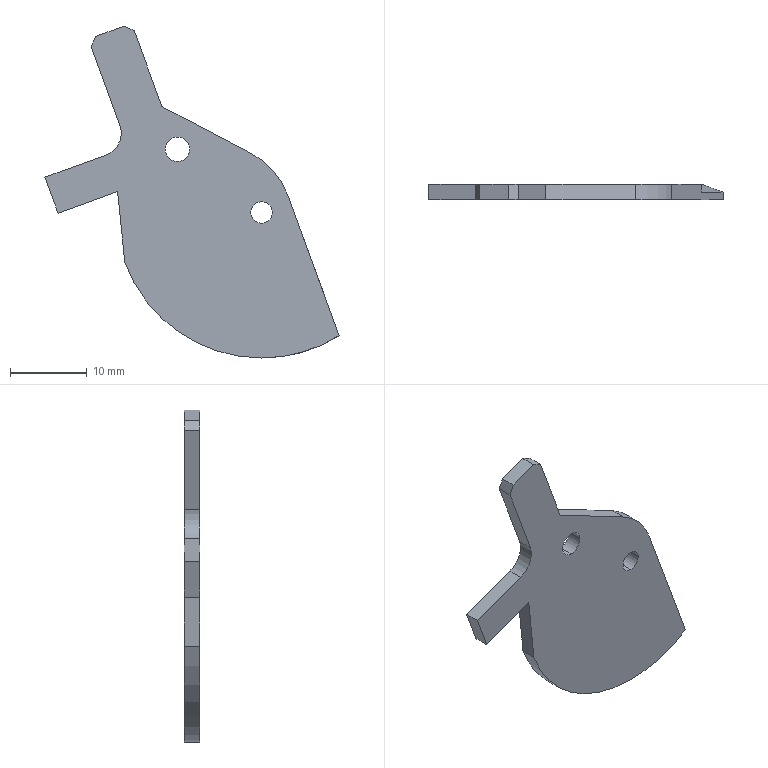Part | SolidWorks | features ICE 14, Fillet 4, Chamfer 3, Extrusion 1 | 1 solid | 23 faces | box 38.392 x 2 x 43.344 mm | volume 1473 mm3 | plane 15 | cylinder 8 | commonest cylinder face diameters 2.8 x2 3.2 x2 38 x2 6 x1 20 x1
STEP:
#1=CARTESIAN_POINT('',(-10.981,0.,6.641));
#2=VERTEX_POINT('',#1);
#3=CARTESIAN_POINT('',(-10.981,0.,9.841));
#4=VERTEX_POINT('',#3);
#5=CARTESIAN_POINT('',(-10.981,0.,8.241));
#6=DIRECTION('',(0.,1.,0.));
#7=DIRECTION('',(0.,0.,1.));
#8=AXIS2_PLACEMENT_3D('',#5,#6,#7);
#9=CIRCLE('',#8,1.6);
#10=EDGE_CURVE('',#2,#4,#9,.T.);
#11=ORIENTED_EDGE('',*,*,#10,.F.);
#12=CARTESIAN_POINT('',(-10.981,2.,6.641));
#13=VERTEX_POINT('',#12);
#14=CARTESIAN_POINT('',(-10.981,-8.,6.641));
#15=DIRECTION('',(0.,1.,0.));
#16=VECTOR('',#15,1000.);
#17=LINE('',#14,#16);
#18=EDGE_CURVE('',#2,#13,#17,.T.);
#19=ORIENTED_EDGE('',*,*,#18,.T.);
#20=CARTESIAN_POINT('',(-10.981,2.,9.841));
#21=VERTEX_POINT('',#20);
#22=CARTESIAN_POINT('',(-10.981,2.,8.241));
#23=DIRECTION('',(0.,1.,0.));
#24=DIRECTION('',(0.,0.,1.));
#25=AXIS2_PLACEMENT_3D('',#22,#23,#24);
#26=CIRCLE('',#25,1.6);
#27=EDGE_CURVE('',#13,#21,#26,.T.);
#28=ORIENTED_EDGE('',*,*,#27,.T.);
#29=CARTESIAN_POINT('',(-10.981,-8.,9.841));
#30=DIRECTION('',(0.,1.,0.));
#31=VECTOR('',#30,1000.);
#32=LINE('',#29,#31);
#33=EDGE_CURVE('',#4,#21,#32,.T.);
#34=ORIENTED_EDGE('',*,*,#33,.F.);
#35=EDGE_LOOP('',(#11,#19,#28,#34));
#36=FACE_OUTER_BOUND('',#35,.T.);
#37=CARTESIAN_POINT('',(-10.981,-8.,8.241));
#38=DIRECTION('',(0.,1.,0.));
#39=DIRECTION('',(0.,0.,1.));
#40=AXIS2_PLACEMENT_3D('',#37,#38,#39);
#41=CYLINDRICAL_SURFACE('',#40,1.6);
#42=ADVANCED_FACE('',(#36),#41,.F.);
#43=CARTESIAN_POINT('',(0.,0.,-1.4));
#44=VERTEX_POINT('',#43);
#45=CARTESIAN_POINT('',(0.,0.,1.4));
#46=VERTEX_POINT('',#45);
#47=CARTESIAN_POINT('',(0.,0.,0.));
#48=DIRECTION('',(0.,1.,0.));
#49=DIRECTION('',(0.,0.,1.));
#50=AXIS2_PLACEMENT_3D('',#47,#48,#49);
#51=CIRCLE('',#50,1.4);
#52=EDGE_CURVE('',#44,#46,#51,.T.);
#53=ORIENTED_EDGE('',*,*,#52,.F.);
#54=CARTESIAN_POINT('',(0.,2.,-1.4));
#55=VERTEX_POINT('',#54);
#56=CARTESIAN_POINT('',(0.,-3.,-1.4));
#57=DIRECTION('',(0.,1.,0.));
#58=VECTOR('',#57,1000.);
#59=LINE('',#56,#58);
#60=EDGE_CURVE('',#44,#55,#59,.T.);
#61=ORIENTED_EDGE('',*,*,#60,.T.);
#62=CARTESIAN_POINT('',(0.,2.,1.4));
#63=VERTEX_POINT('',#62);
#64=CARTESIAN_POINT('',(0.,2.,0.));
#65=DIRECTION('',(0.,1.,0.));
#66=DIRECTION('',(0.,0.,1.));
#67=AXIS2_PLACEMENT_3D('',#64,#65,#66);
#68=CIRCLE('',#67,1.4);
#69=EDGE_CURVE('',#55,#63,#68,.T.);
#70=ORIENTED_EDGE('',*,*,#69,.T.);
#71=CARTESIAN_POINT('',(0.,-3.,1.4));
#72=DIRECTION('',(0.,1.,0.));
#73=VECTOR('',#72,1000.);
#74=LINE('',#71,#73);
#75=EDGE_CURVE('',#46,#63,#74,.T.);
#76=ORIENTED_EDGE('',*,*,#75,.F.);
#77=EDGE_LOOP('',(#53,#61,#70,#76));
#78=FACE_OUTER_BOUND('',#77,.T.);
#79=CARTESIAN_POINT('',(0.,-3.,0.));
#80=DIRECTION('',(0.,1.,0.));
#81=DIRECTION('',(0.,0.,1.));
#82=AXIS2_PLACEMENT_3D('',#79,#80,#81);
#83=CYLINDRICAL_SURFACE('',#82,1.4);
#84=ADVANCED_FACE('',(#78),#83,.F.);
#85=CARTESIAN_POINT('',(0.,2.,-19.));
#86=VERTEX_POINT('',#85);
#87=CARTESIAN_POINT('',(-17.854,2.,-6.498));
#88=VERTEX_POINT('',#87);
#89=CARTESIAN_POINT('',(0.,2.,0.));
#90=DIRECTION('',(0.,1.,0.));
#91=DIRECTION('',(0.,0.,1.));
#92=AXIS2_PLACEMENT_3D('',#89,#90,#91);
#93=CIRCLE('',#92,19.);
#94=EDGE_CURVE('',#86,#88,#93,.T.);
#95=ORIENTED_EDGE('',*,*,#94,.F.);
#96=CARTESIAN_POINT('',(0.,0.,-19.));
#97=VERTEX_POINT('',#96);
#98=CARTESIAN_POINT('',(0.,2.,-19.));
#99=DIRECTION('',(0.,-1.,0.));
#100=VECTOR('',#99,1000.);
#101=LINE('',#98,#100);
#102=EDGE_CURVE('',#86,#97,#101,.T.);
#103=ORIENTED_EDGE('',*,*,#102,.T.);
#104=CARTESIAN_POINT('',(-17.854,0.,-6.498));
#105=VERTEX_POINT('',#104);
#106=CARTESIAN_POINT('',(0.,0.,0.));
#107=DIRECTION('',(0.,1.,0.));
#108=DIRECTION('',(0.,0.,1.));
#109=AXIS2_PLACEMENT_3D('',#106,#107,#108);
#110=CIRCLE('',#109,19.);
#111=EDGE_CURVE('',#97,#105,#110,.T.);
#112=ORIENTED_EDGE('',*,*,#111,.T.);
#113=CARTESIAN_POINT('',(-17.854,-8.,-6.498));
#114=DIRECTION('',(0.,1.,0.));
#115=VECTOR('',#114,1000.);
#116=LINE('',#113,#115);
#117=EDGE_CURVE('',#105,#88,#116,.T.);
#118=ORIENTED_EDGE('',*,*,#117,.T.);
#119=EDGE_LOOP('',(#95,#103,#112,#118));
#120=FACE_OUTER_BOUND('',#119,.T.);
#121=CARTESIAN_POINT('',(0.,2.,0.));
#122=DIRECTION('',(0.,-1.,0.));
#123=DIRECTION('',(0.,0.,-1.));
#124=AXIS2_PLACEMENT_3D('',#121,#122,#123);
#125=CYLINDRICAL_SURFACE('',#124,19.);
#126=ADVANCED_FACE('',(#120),#125,.T.);
#127=ORIENTED_EDGE('',*,*,#102,.F.);
#128=CARTESIAN_POINT('',(7.429,2.,-17.487));
#129=VERTEX_POINT('',#128);
#130=CARTESIAN_POINT('',(0.,2.,0.));
#131=DIRECTION('',(0.,1.,0.));
#132=DIRECTION('',(0.,0.,1.));
#133=AXIS2_PLACEMENT_3D('',#130,#131,#132);
#134=CIRCLE('',#133,19.);
#135=EDGE_CURVE('',#129,#86,#134,.T.);
#136=ORIENTED_EDGE('',*,*,#135,.F.);
#137=CARTESIAN_POINT('',(10.112,1.,-16.086));
#138=VERTEX_POINT('',#137);
#139=CARTESIAN_POINT('',(7.429,2.,-17.487));
#140=CARTESIAN_POINT('',(8.36,1.663,-17.092));
#141=CARTESIAN_POINT('',(9.256,1.329,-16.624));
#142=CARTESIAN_POINT('',(10.112,1.,-16.086));
#143=(BOUNDED_CURVE()B_SPLINE_CURVE(3,(#139,#140,#141,#142),.UNSPECIFIED.,.F.,.F.)B_SPLINE_CURVE_WITH_KNOTS((4,4),(4.765,4.925),.UNSPECIFIED.)CURVE()GEOMETRIC_REPRESENTATION_ITEM()RATIONAL_B_SPLINE_CURVE((1.,0.9979,0.9979,1.))REPRESENTATION_ITEM(''));
#144=EDGE_CURVE('',#129,#138,#143,.T.);
#145=ORIENTED_EDGE('',*,*,#144,.T.);
#146=CARTESIAN_POINT('',(10.112,0.,-16.086));
#147=VERTEX_POINT('',#146);
#148=CARTESIAN_POINT('',(10.112,2.,-16.086));
#149=DIRECTION('',(0.,-1.,0.));
#150=VECTOR('',#149,1000.);
#151=LINE('',#148,#150);
#152=EDGE_CURVE('',#138,#147,#151,.T.);
#153=ORIENTED_EDGE('',*,*,#152,.T.);
#154=CARTESIAN_POINT('',(0.,0.,0.));
#155=DIRECTION('',(0.,1.,0.));
#156=DIRECTION('',(0.,0.,1.));
#157=AXIS2_PLACEMENT_3D('',#154,#155,#156);
#158=CIRCLE('',#157,19.);
#159=EDGE_CURVE('',#147,#97,#158,.T.);
#160=ORIENTED_EDGE('',*,*,#159,.T.);
#161=EDGE_LOOP('',(#127,#136,#145,#153,#160));
#162=FACE_OUTER_BOUND('',#161,.T.);
#163=CARTESIAN_POINT('',(0.,2.,0.));
#164=DIRECTION('',(0.,-1.,0.));
#165=DIRECTION('',(0.,0.,-1.));
#166=AXIS2_PLACEMENT_3D('',#163,#164,#165);
#167=CYLINDRICAL_SURFACE('',#166,19.);
#168=ADVANCED_FACE('',(#162),#167,.T.);
#169=CARTESIAN_POINT('',(-10.981,2.,8.241));
#170=DIRECTION('',(0.,1.,0.));
#171=DIRECTION('',(0.,0.,1.));
#172=AXIS2_PLACEMENT_3D('',#169,#170,#171);
#173=CIRCLE('',#172,1.6);
#174=EDGE_CURVE('',#21,#13,#173,.T.);
#175=ORIENTED_EDGE('',*,*,#174,.F.);
#176=ORIENTED_EDGE('',*,*,#27,.F.);
#177=EDGE_LOOP('',(#175,#176));
#178=FACE_BOUND('',#177,.T.);
#179=CARTESIAN_POINT('',(-21.665,2.,22.976));
#180=VERTEX_POINT('',#179);
#181=CARTESIAN_POINT('',(-17.906,2.,24.344));
#182=VERTEX_POINT('',#181);
#183=CARTESIAN_POINT('',(-16.966,2.,24.686));
#184=DIRECTION('',(0.9397,0.,0.342));
#185=VECTOR('',#184,1000.);
#186=LINE('',#183,#185);
#187=EDGE_CURVE('',#180,#182,#186,.T.);
#188=ORIENTED_EDGE('',*,*,#187,.T.);
#189=CARTESIAN_POINT('',(-16.624,2.,23.746));
#190=VERTEX_POINT('',#189);
#191=CARTESIAN_POINT('',(6.126,2.,13.138));
#192=DIRECTION('',(0.9063,0.,-0.4226));
#193=VECTOR('',#192,1000.);
#194=LINE('',#191,#193);
#195=EDGE_CURVE('',#182,#190,#194,.T.);
#196=ORIENTED_EDGE('',*,*,#195,.T.);
#197=CARTESIAN_POINT('',(-13.018,2.,13.839));
#198=VERTEX_POINT('',#197);
#199=CARTESIAN_POINT('',(-10.126,2.,5.892));
#200=DIRECTION('',(0.342,0.,-0.9397));
#201=VECTOR('',#200,1000.);
#202=LINE('',#199,#201);
#203=EDGE_CURVE('',#190,#198,#202,.T.);
#204=ORIENTED_EDGE('',*,*,#203,.T.);
#205=CARTESIAN_POINT('',(-1.306,2.,7.682));
#206=VERTEX_POINT('',#205);
#207=CARTESIAN_POINT('',(-13.018,2.,13.839));
#208=DIRECTION('',(-0.8851,0.,0.4653));
#209=VECTOR('',#208,1000.);
#210=LINE('',#207,#209);
#211=EDGE_CURVE('',#206,#198,#210,.T.);
#212=ORIENTED_EDGE('',*,*,#211,.F.);
#213=CARTESIAN_POINT('',(3.437,2.,2.251));
#214=VERTEX_POINT('',#213);
#215=CARTESIAN_POINT('',(-5.96,2.,-1.169));
#216=DIRECTION('',(0.,1.,0.));
#217=DIRECTION('',(0.,0.,1.));
#218=AXIS2_PLACEMENT_3D('',#215,#216,#217);
#219=CIRCLE('',#218,10.);
#220=EDGE_CURVE('',#206,#214,#219,.T.);
#221=ORIENTED_EDGE('',*,*,#220,.T.);
#222=CARTESIAN_POINT('',(7.261,2.,-8.256));
#223=VERTEX_POINT('',#222);
#224=CARTESIAN_POINT('',(-2.999,2.,19.935));
#225=DIRECTION('',(0.342,0.,-0.9397));
#226=VECTOR('',#225,1000.);
#227=LINE('',#224,#226);
#228=EDGE_CURVE('',#214,#223,#227,.T.);
#229=ORIENTED_EDGE('',*,*,#228,.T.);
#230=CARTESIAN_POINT('',(4.442,2.,-9.282));
#231=VERTEX_POINT('',#230);
#232=CARTESIAN_POINT('',(7.261,2.,-8.256));
#233=DIRECTION('',(-0.9397,0.,-0.342));
#234=VECTOR('',#233,1000.);
#235=LINE('',#232,#234);
#236=EDGE_CURVE('',#223,#231,#235,.T.);
#237=ORIENTED_EDGE('',*,*,#236,.T.);
#238=CARTESIAN_POINT('',(7.292,2.,-17.112));
#239=DIRECTION('',(0.342,0.,-0.9397));
#240=VECTOR('',#239,1000.);
#241=LINE('',#238,#240);
#242=EDGE_CURVE('',#231,#129,#241,.T.);
#243=ORIENTED_EDGE('',*,*,#242,.T.);
#244=ORIENTED_EDGE('',*,*,#135,.T.);
#245=ORIENTED_EDGE('',*,*,#94,.T.);
#246=CARTESIAN_POINT('',(-18.802,2.,2.734));
#247=VERTEX_POINT('',#246);
#248=CARTESIAN_POINT('',(-18.802,2.,2.734));
#249=DIRECTION('',(0.1022,0.,-0.9948));
#250=VECTOR('',#249,1000.);
#251=LINE('',#248,#250);
#252=EDGE_CURVE('',#247,#88,#251,.T.);
#253=ORIENTED_EDGE('',*,*,#252,.F.);
#254=CARTESIAN_POINT('',(-26.57,2.,-0.09327));
#255=VERTEX_POINT('',#254);
#256=CARTESIAN_POINT('',(-26.57,2.,-0.09327));
#257=DIRECTION('',(-0.9397,0.,-0.342));
#258=VECTOR('',#257,1000.);
#259=LINE('',#256,#258);
#260=EDGE_CURVE('',#247,#255,#259,.T.);
#261=ORIENTED_EDGE('',*,*,#260,.T.);
#262=CARTESIAN_POINT('',(-28.281,2.,4.605));
#263=VERTEX_POINT('',#262);
#264=CARTESIAN_POINT('',(-28.281,2.,4.605));
#265=DIRECTION('',(-0.342,0.,0.9397));
#266=VECTOR('',#265,1000.);
#267=LINE('',#264,#266);
#268=EDGE_CURVE('',#255,#263,#267,.T.);
#269=ORIENTED_EDGE('',*,*,#268,.T.);
#270=CARTESIAN_POINT('',(-20.293,2.,7.512));
#271=VERTEX_POINT('',#270);
#272=CARTESIAN_POINT('',(-17.474,2.,8.538));
#273=DIRECTION('',(0.9397,0.,0.342));
#274=VECTOR('',#273,1000.);
#275=LINE('',#272,#274);
#276=EDGE_CURVE('',#263,#271,#275,.T.);
#277=ORIENTED_EDGE('',*,*,#276,.T.);
#278=CARTESIAN_POINT('',(-18.5,2.,11.358));
#279=VERTEX_POINT('',#278);
#280=CARTESIAN_POINT('',(-21.319,2.,10.331));
#281=DIRECTION('',(0.,-1.,0.));
#282=DIRECTION('',(0.,0.,1.));
#283=AXIS2_PLACEMENT_3D('',#280,#281,#282);
#284=CIRCLE('',#283,3.);
#285=EDGE_CURVE('',#271,#279,#284,.T.);
#286=ORIENTED_EDGE('',*,*,#285,.T.);
#287=CARTESIAN_POINT('',(-22.262,2.,21.694));
#288=VERTEX_POINT('',#287);
#289=CARTESIAN_POINT('',(-22.604,2.,22.634));
#290=DIRECTION('',(-0.342,0.,0.9397));
#291=VECTOR('',#290,1000.);
#292=LINE('',#289,#291);
#293=EDGE_CURVE('',#279,#288,#292,.T.);
#294=ORIENTED_EDGE('',*,*,#293,.T.);
#295=CARTESIAN_POINT('',(-26.596,2.,12.402));
#296=DIRECTION('',(0.4226,0.,0.9063));
#297=VECTOR('',#296,1000.);
#298=LINE('',#295,#297);
#299=EDGE_CURVE('',#288,#180,#298,.T.);
#300=ORIENTED_EDGE('',*,*,#299,.T.);
#301=EDGE_LOOP('',(#188,#196,#204,#212,#221,#229,#237,#243,#244,#245,#253,#261,#269,#277,#286,#294,#300));
#302=FACE_OUTER_BOUND('',#301,.T.);
#303=CARTESIAN_POINT('',(0.,2.,0.));
#304=DIRECTION('',(0.,1.,0.));
#305=DIRECTION('',(0.,0.,1.));
#306=AXIS2_PLACEMENT_3D('',#303,#304,#305);
#307=CIRCLE('',#306,1.4);
#308=EDGE_CURVE('',#63,#55,#307,.T.);
#309=ORIENTED_EDGE('',*,*,#308,.F.);
#310=ORIENTED_EDGE('',*,*,#69,.F.);
#311=EDGE_LOOP('',(#309,#310));
#312=FACE_BOUND('',#311,.T.);
#313=CARTESIAN_POINT('',(0.,2.,0.));
#314=DIRECTION('',(0.,1.,0.));
#315=DIRECTION('',(0.,0.,1.));
#316=AXIS2_PLACEMENT_3D('',#313,#314,#315);
#317=PLANE('',#316);
#318=ADVANCED_FACE('',(#178,#302,#312),#317,.T.);
#319=CARTESIAN_POINT('',(-10.981,0.,8.241));
#320=DIRECTION('',(0.,1.,0.));
#321=DIRECTION('',(0.,0.,1.));
#322=AXIS2_PLACEMENT_3D('',#319,#320,#321);
#323=CIRCLE('',#322,1.6);
#324=EDGE_CURVE('',#4,#2,#323,.T.);
#325=ORIENTED_EDGE('',*,*,#324,.T.);
#326=ORIENTED_EDGE('',*,*,#10,.T.);
#327=EDGE_LOOP('',(#325,#326));
#328=FACE_BOUND('',#327,.T.);
#329=CARTESIAN_POINT('',(-13.018,0.,13.839));
#330=VERTEX_POINT('',#329);
#331=CARTESIAN_POINT('',(-16.624,0.,23.746));
#332=VERTEX_POINT('',#331);
#333=CARTESIAN_POINT('',(-10.126,0.,5.892));
#334=DIRECTION('',(-0.342,0.,0.9397));
#335=VECTOR('',#334,1000.);
#336=LINE('',#333,#335);
#337=EDGE_CURVE('',#330,#332,#336,.T.);
#338=ORIENTED_EDGE('',*,*,#337,.T.);
#339=CARTESIAN_POINT('',(-17.906,0.,24.344));
#340=VERTEX_POINT('',#339);
#341=CARTESIAN_POINT('',(-17.906,0.,24.344));
#342=DIRECTION('',(-0.9063,0.,0.4226));
#343=VECTOR('',#342,1000.);
#344=LINE('',#341,#343);
#345=EDGE_CURVE('',#332,#340,#344,.T.);
#346=ORIENTED_EDGE('',*,*,#345,.T.);
#347=CARTESIAN_POINT('',(-21.665,0.,22.976));
#348=VERTEX_POINT('',#347);
#349=CARTESIAN_POINT('',(-16.966,0.,24.686));
#350=DIRECTION('',(-0.9397,0.,-0.342));
#351=VECTOR('',#350,1000.);
#352=LINE('',#349,#351);
#353=EDGE_CURVE('',#340,#348,#352,.T.);
#354=ORIENTED_EDGE('',*,*,#353,.T.);
#355=CARTESIAN_POINT('',(-22.262,0.,21.694));
#356=VERTEX_POINT('',#355);
#357=CARTESIAN_POINT('',(-22.262,0.,21.694));
#358=DIRECTION('',(-0.4226,0.,-0.9063));
#359=VECTOR('',#358,1000.);
#360=LINE('',#357,#359);
#361=EDGE_CURVE('',#348,#356,#360,.T.);
#362=ORIENTED_EDGE('',*,*,#361,.T.);
#363=CARTESIAN_POINT('',(-18.5,0.,11.358));
#364=VERTEX_POINT('',#363);
#365=CARTESIAN_POINT('',(-22.604,0.,22.634));
#366=DIRECTION('',(0.342,0.,-0.9397));
#367=VECTOR('',#366,1000.);
#368=LINE('',#365,#367);
#369=EDGE_CURVE('',#356,#364,#368,.T.);
#370=ORIENTED_EDGE('',*,*,#369,.T.);
#371=CARTESIAN_POINT('',(-20.293,0.,7.512));
#372=VERTEX_POINT('',#371);
#373=CARTESIAN_POINT('',(-21.319,0.,10.331));
#374=DIRECTION('',(0.,1.,0.));
#375=DIRECTION('',(0.,0.,1.));
#376=AXIS2_PLACEMENT_3D('',#373,#374,#375);
#377=CIRCLE('',#376,3.);
#378=EDGE_CURVE('',#364,#372,#377,.T.);
#379=ORIENTED_EDGE('',*,*,#378,.T.);
#380=CARTESIAN_POINT('',(-28.281,0.,4.605));
#381=VERTEX_POINT('',#380);
#382=CARTESIAN_POINT('',(-17.474,0.,8.538));
#383=DIRECTION('',(-0.9397,0.,-0.342));
#384=VECTOR('',#383,1000.);
#385=LINE('',#382,#384);
#386=EDGE_CURVE('',#372,#381,#385,.T.);
#387=ORIENTED_EDGE('',*,*,#386,.T.);
#388=CARTESIAN_POINT('',(-26.57,0.,-0.09327));
#389=VERTEX_POINT('',#388);
#390=CARTESIAN_POINT('',(-28.281,0.,4.605));
#391=DIRECTION('',(0.342,0.,-0.9397));
#392=VECTOR('',#391,1000.);
#393=LINE('',#390,#392);
#394=EDGE_CURVE('',#381,#389,#393,.T.);
#395=ORIENTED_EDGE('',*,*,#394,.T.);
#396=CARTESIAN_POINT('',(-18.802,0.,2.734));
#397=VERTEX_POINT('',#396);
#398=CARTESIAN_POINT('',(-26.57,0.,-0.09327));
#399=DIRECTION('',(0.9397,0.,0.342));
#400=VECTOR('',#399,1000.);
#401=LINE('',#398,#400);
#402=EDGE_CURVE('',#389,#397,#401,.T.);
#403=ORIENTED_EDGE('',*,*,#402,.T.);
#404=CARTESIAN_POINT('',(-18.328,0.,-1.882));
#405=DIRECTION('',(0.1022,0.,-0.9948));
#406=VECTOR('',#405,1000.);
#407=LINE('',#404,#406);
#408=EDGE_CURVE('',#397,#105,#407,.T.);
#409=ORIENTED_EDGE('',*,*,#408,.T.);
#410=ORIENTED_EDGE('',*,*,#111,.F.);
#411=ORIENTED_EDGE('',*,*,#159,.F.);
#412=CARTESIAN_POINT('',(3.437,0.,2.251));
#413=VERTEX_POINT('',#412);
#414=CARTESIAN_POINT('',(3.759,0.,1.368));
#415=DIRECTION('',(-0.342,0.,0.9397));
#416=VECTOR('',#415,1000.);
#417=LINE('',#414,#416);
#418=EDGE_CURVE('',#147,#413,#417,.T.);
#419=ORIENTED_EDGE('',*,*,#418,.T.);
#420=CARTESIAN_POINT('',(-1.306,0.,7.682));
#421=VERTEX_POINT('',#420);
#422=CARTESIAN_POINT('',(-5.96,0.,-1.169));
#423=DIRECTION('',(0.,-1.,0.));
#424=DIRECTION('',(0.,0.,1.));
#425=AXIS2_PLACEMENT_3D('',#422,#423,#424);
#426=CIRCLE('',#425,10.);
#427=EDGE_CURVE('',#413,#421,#426,.T.);
#428=ORIENTED_EDGE('',*,*,#427,.T.);
#429=CARTESIAN_POINT('',(2.881,0.,5.481));
#430=DIRECTION('',(-0.8851,0.,0.4653));
#431=VECTOR('',#430,1000.);
#432=LINE('',#429,#431);
#433=EDGE_CURVE('',#421,#330,#432,.T.);
#434=ORIENTED_EDGE('',*,*,#433,.T.);
#435=EDGE_LOOP('',(#338,#346,#354,#362,#370,#379,#387,#395,#403,#409,#410,#411,#419,#428,#434));
#436=FACE_OUTER_BOUND('',#435,.T.);
#437=CARTESIAN_POINT('',(0.,0.,0.));
#438=DIRECTION('',(0.,1.,0.));
#439=DIRECTION('',(0.,0.,1.));
#440=AXIS2_PLACEMENT_3D('',#437,#438,#439);
#441=CIRCLE('',#440,1.4);
#442=EDGE_CURVE('',#46,#44,#441,.T.);
#443=ORIENTED_EDGE('',*,*,#442,.T.);
#444=ORIENTED_EDGE('',*,*,#52,.T.);
#445=EDGE_LOOP('',(#443,#444));
#446=FACE_BOUND('',#445,.T.);
#447=CARTESIAN_POINT('',(0.,0.,0.));
#448=DIRECTION('',(0.,1.,0.));
#449=DIRECTION('',(0.,0.,1.));
#450=AXIS2_PLACEMENT_3D('',#447,#448,#449);
#451=PLANE('',#450);
#452=ADVANCED_FACE('',(#328,#436,#446),#451,.F.);
#453=ORIENTED_EDGE('',*,*,#228,.F.);
#454=CARTESIAN_POINT('',(3.437,-3.,2.251));
#455=DIRECTION('',(0.,-1.,0.));
#456=VECTOR('',#455,1000.);
#457=LINE('',#454,#456);
#458=EDGE_CURVE('',#214,#413,#457,.T.);
#459=ORIENTED_EDGE('',*,*,#458,.T.);
#460=ORIENTED_EDGE('',*,*,#418,.F.);
#461=ORIENTED_EDGE('',*,*,#152,.F.);
#462=CARTESIAN_POINT('',(7.261,1.,-8.256));
#463=VERTEX_POINT('',#462);
#464=CARTESIAN_POINT('',(-2.999,1.,19.935));
#465=DIRECTION('',(-0.342,0.,0.9397));
#466=VECTOR('',#465,1000.);
#467=LINE('',#464,#466);
#468=EDGE_CURVE('',#138,#463,#467,.T.);
#469=ORIENTED_EDGE('',*,*,#468,.T.);
#470=CARTESIAN_POINT('',(7.261,-32.011,-8.256));
#471=DIRECTION('',(0.,1.,0.));
#472=VECTOR('',#471,1000.);
#473=LINE('',#470,#472);
#474=EDGE_CURVE('',#463,#223,#473,.T.);
#475=ORIENTED_EDGE('',*,*,#474,.T.);
#476=EDGE_LOOP('',(#453,#459,#460,#461,#469,#475));
#477=FACE_OUTER_BOUND('',#476,.T.);
#478=CARTESIAN_POINT('',(11.93,-3.,-21.083));
#479=DIRECTION('',(-0.9397,0.,-0.342));
#480=DIRECTION('',(-0.342,0.,0.9397));
#481=AXIS2_PLACEMENT_3D('',#478,#479,#480);
#482=PLANE('',#481);
#483=ADVANCED_FACE('',(#477),#482,.F.);
#484=ORIENTED_EDGE('',*,*,#60,.F.);
#485=ORIENTED_EDGE('',*,*,#442,.F.);
#486=ORIENTED_EDGE('',*,*,#75,.T.);
#487=ORIENTED_EDGE('',*,*,#308,.T.);
#488=EDGE_LOOP('',(#484,#485,#486,#487));
#489=FACE_OUTER_BOUND('',#488,.T.);
#490=CARTESIAN_POINT('',(0.,-3.,0.));
#491=DIRECTION('',(0.,1.,0.));
#492=DIRECTION('',(0.,0.,1.));
#493=AXIS2_PLACEMENT_3D('',#490,#491,#492);
#494=CYLINDRICAL_SURFACE('',#493,1.4);
#495=ADVANCED_FACE('',(#489),#494,.F.);
#496=CARTESIAN_POINT('',(7.261,1.,-8.256));
#497=DIRECTION('',(-0.8915,0.3162,-0.3245));
#498=VECTOR('',#497,1000.);
#499=LINE('',#496,#498);
#500=EDGE_CURVE('',#463,#231,#499,.T.);
#501=ORIENTED_EDGE('',*,*,#500,.F.);
#502=ORIENTED_EDGE('',*,*,#468,.F.);
#503=ORIENTED_EDGE('',*,*,#144,.F.);
#504=ORIENTED_EDGE('',*,*,#242,.F.);
#505=EDGE_LOOP('',(#501,#502,#503,#504));
#506=FACE_OUTER_BOUND('',#505,.T.);
#507=CARTESIAN_POINT('',(11.93,1.,-21.083));
#508=DIRECTION('',(0.2972,0.9487,0.1082));
#509=DIRECTION('',(0.342,0.,-0.9397));
#510=AXIS2_PLACEMENT_3D('',#507,#508,#509);
#511=PLANE('',#510);
#512=ADVANCED_FACE('',(#506),#511,.T.);
#513=ORIENTED_EDGE('',*,*,#474,.F.);
#514=ORIENTED_EDGE('',*,*,#500,.T.);
#515=ORIENTED_EDGE('',*,*,#236,.F.);
#516=EDGE_LOOP('',(#513,#514,#515));
#517=FACE_OUTER_BOUND('',#516,.T.);
#518=CARTESIAN_POINT('',(7.261,-32.011,-8.256));
#519=DIRECTION('',(0.342,0.,-0.9397));
#520=DIRECTION('',(-0.9397,0.,-0.342));
#521=AXIS2_PLACEMENT_3D('',#518,#519,#520);
#522=PLANE('',#521);
#523=ADVANCED_FACE('',(#517),#522,.T.);
#524=CARTESIAN_POINT('',(-18.802,2.,2.734));
#525=DIRECTION('',(0.,1.,0.));
#526=VECTOR('',#525,1000.);
#527=LINE('',#524,#526);
#528=EDGE_CURVE('',#397,#247,#527,.T.);
#529=ORIENTED_EDGE('',*,*,#528,.F.);
#530=ORIENTED_EDGE('',*,*,#402,.F.);
#531=CARTESIAN_POINT('',(-26.57,-30.718,-0.09327));
#532=DIRECTION('',(0.,1.,0.));
#533=VECTOR('',#532,1000.);
#534=LINE('',#531,#533);
#535=EDGE_CURVE('',#389,#255,#534,.T.);
#536=ORIENTED_EDGE('',*,*,#535,.T.);
#537=ORIENTED_EDGE('',*,*,#260,.F.);
#538=EDGE_LOOP('',(#529,#530,#536,#537));
#539=FACE_OUTER_BOUND('',#538,.T.);
#540=CARTESIAN_POINT('',(-26.57,-30.718,-0.09327));
#541=DIRECTION('',(0.342,0.,-0.9397));
#542=DIRECTION('',(-0.9397,0.,-0.342));
#543=AXIS2_PLACEMENT_3D('',#540,#541,#542);
#544=PLANE('',#543);
#545=ADVANCED_FACE('',(#539),#544,.T.);
#546=ORIENTED_EDGE('',*,*,#203,.F.);
#547=CARTESIAN_POINT('',(-16.624,-30.718,23.746));
#548=DIRECTION('',(0.,-1.,0.));
#549=VECTOR('',#548,1000.);
#550=LINE('',#547,#549);
#551=EDGE_CURVE('',#190,#332,#550,.T.);
#552=ORIENTED_EDGE('',*,*,#551,.T.);
#553=ORIENTED_EDGE('',*,*,#337,.F.);
#554=CARTESIAN_POINT('',(-13.018,2.,13.839));
#555=DIRECTION('',(0.,-1.,0.));
#556=VECTOR('',#555,1000.);
#557=LINE('',#554,#556);
#558=EDGE_CURVE('',#198,#330,#557,.T.);
#559=ORIENTED_EDGE('',*,*,#558,.F.);
#560=EDGE_LOOP('',(#546,#552,#553,#559));
#561=FACE_OUTER_BOUND('',#560,.T.);
#562=CARTESIAN_POINT('',(-10.126,-30.718,5.892));
#563=DIRECTION('',(0.9397,0.,0.342));
#564=DIRECTION('',(0.342,0.,-0.9397));
#565=AXIS2_PLACEMENT_3D('',#562,#563,#564);
#566=PLANE('',#565);
#567=ADVANCED_FACE('',(#561),#566,.T.);
#568=ORIENTED_EDGE('',*,*,#353,.F.);
#569=CARTESIAN_POINT('',(-17.906,-30.718,24.344));
#570=DIRECTION('',(0.,1.,0.));
#571=VECTOR('',#570,1000.);
#572=LINE('',#569,#571);
#573=EDGE_CURVE('',#340,#182,#572,.T.);
#574=ORIENTED_EDGE('',*,*,#573,.T.);
#575=ORIENTED_EDGE('',*,*,#187,.F.);
#576=CARTESIAN_POINT('',(-21.665,-30.718,22.976));
#577=DIRECTION('',(0.,-1.,0.));
#578=VECTOR('',#577,1000.);
#579=LINE('',#576,#578);
#580=EDGE_CURVE('',#180,#348,#579,.T.);
#581=ORIENTED_EDGE('',*,*,#580,.T.);
#582=EDGE_LOOP('',(#568,#574,#575,#581));
#583=FACE_OUTER_BOUND('',#582,.T.);
#584=CARTESIAN_POINT('',(-16.966,-30.718,24.686));
#585=DIRECTION('',(-0.342,0.,0.9397));
#586=DIRECTION('',(0.9397,0.,0.342));
#587=AXIS2_PLACEMENT_3D('',#584,#585,#586);
#588=PLANE('',#587);
#589=ADVANCED_FACE('',(#583),#588,.T.);
#590=ORIENTED_EDGE('',*,*,#293,.F.);
#591=CARTESIAN_POINT('',(-18.5,0.,11.358));
#592=DIRECTION('',(0.,-1.,0.));
#593=VECTOR('',#592,1000.);
#594=LINE('',#591,#593);
#595=EDGE_CURVE('',#279,#364,#594,.T.);
#596=ORIENTED_EDGE('',*,*,#595,.T.);
#597=ORIENTED_EDGE('',*,*,#369,.F.);
#598=CARTESIAN_POINT('',(-22.262,-30.718,21.694));
#599=DIRECTION('',(0.,1.,0.));
#600=VECTOR('',#599,1000.);
#601=LINE('',#598,#600);
#602=EDGE_CURVE('',#356,#288,#601,.T.);
#603=ORIENTED_EDGE('',*,*,#602,.T.);
#604=EDGE_LOOP('',(#590,#596,#597,#603));
#605=FACE_OUTER_BOUND('',#604,.T.);
#606=CARTESIAN_POINT('',(-22.604,-30.718,22.634));
#607=DIRECTION('',(-0.9397,0.,-0.342));
#608=DIRECTION('',(-0.342,0.,0.9397));
#609=AXIS2_PLACEMENT_3D('',#606,#607,#608);
#610=PLANE('',#609);
#611=ADVANCED_FACE('',(#605),#610,.T.);
#612=ORIENTED_EDGE('',*,*,#386,.F.);
#613=CARTESIAN_POINT('',(-20.293,2.,7.512));
#614=DIRECTION('',(0.,1.,0.));
#615=VECTOR('',#614,1000.);
#616=LINE('',#613,#615);
#617=EDGE_CURVE('',#372,#271,#616,.T.);
#618=ORIENTED_EDGE('',*,*,#617,.T.);
#619=ORIENTED_EDGE('',*,*,#276,.F.);
#620=CARTESIAN_POINT('',(-28.281,-30.718,4.605));
#621=DIRECTION('',(0.,1.,0.));
#622=VECTOR('',#621,1000.);
#623=LINE('',#620,#622);
#624=EDGE_CURVE('',#381,#263,#623,.T.);
#625=ORIENTED_EDGE('',*,*,#624,.F.);
#626=EDGE_LOOP('',(#612,#618,#619,#625));
#627=FACE_OUTER_BOUND('',#626,.T.);
#628=CARTESIAN_POINT('',(-17.474,-30.718,8.538));
#629=DIRECTION('',(-0.342,0.,0.9397));
#630=DIRECTION('',(0.9397,0.,0.342));
#631=AXIS2_PLACEMENT_3D('',#628,#629,#630);
#632=PLANE('',#631);
#633=ADVANCED_FACE('',(#627),#632,.T.);
#634=ORIENTED_EDGE('',*,*,#394,.F.);
#635=ORIENTED_EDGE('',*,*,#624,.T.);
#636=ORIENTED_EDGE('',*,*,#268,.F.);
#637=ORIENTED_EDGE('',*,*,#535,.F.);
#638=EDGE_LOOP('',(#634,#635,#636,#637));
#639=FACE_OUTER_BOUND('',#638,.T.);
#640=CARTESIAN_POINT('',(-28.281,-30.718,4.605));
#641=DIRECTION('',(-0.9397,0.,-0.342));
#642=DIRECTION('',(-0.342,0.,0.9397));
#643=AXIS2_PLACEMENT_3D('',#640,#641,#642);
#644=PLANE('',#643);
#645=ADVANCED_FACE('',(#639),#644,.T.);
#646=ORIENTED_EDGE('',*,*,#433,.F.);
#647=CARTESIAN_POINT('',(-1.306,-8.,7.682));
#648=DIRECTION('',(0.,1.,0.));
#649=VECTOR('',#648,1000.);
#650=LINE('',#647,#649);
#651=EDGE_CURVE('',#421,#206,#650,.T.);
#652=ORIENTED_EDGE('',*,*,#651,.T.);
#653=ORIENTED_EDGE('',*,*,#211,.T.);
#654=ORIENTED_EDGE('',*,*,#558,.T.);
#655=EDGE_LOOP('',(#646,#652,#653,#654));
#656=FACE_OUTER_BOUND('',#655,.T.);
#657=CARTESIAN_POINT('',(-13.018,-8.,13.839));
#658=DIRECTION('',(-0.4653,0.,-0.8851));
#659=DIRECTION('',(-0.8851,0.,0.4653));
#660=AXIS2_PLACEMENT_3D('',#657,#658,#659);
#661=PLANE('',#660);
#662=ADVANCED_FACE('',(#656),#661,.F.);
#663=ORIENTED_EDGE('',*,*,#528,.T.);
#664=ORIENTED_EDGE('',*,*,#252,.T.);
#665=ORIENTED_EDGE('',*,*,#117,.F.);
#666=ORIENTED_EDGE('',*,*,#408,.F.);
#667=EDGE_LOOP('',(#663,#664,#665,#666));
#668=FACE_OUTER_BOUND('',#667,.T.);
#669=CARTESIAN_POINT('',(-18.802,-8.,2.734));
#670=DIRECTION('',(0.9948,0.,0.1022));
#671=DIRECTION('',(0.1022,0.,-0.9948));
#672=AXIS2_PLACEMENT_3D('',#669,#670,#671);
#673=PLANE('',#672);
#674=ADVANCED_FACE('',(#668),#673,.F.);
#675=ORIENTED_EDGE('',*,*,#427,.F.);
#676=ORIENTED_EDGE('',*,*,#458,.F.);
#677=ORIENTED_EDGE('',*,*,#220,.F.);
#678=ORIENTED_EDGE('',*,*,#651,.F.);
#679=EDGE_LOOP('',(#675,#676,#677,#678));
#680=FACE_OUTER_BOUND('',#679,.T.);
#681=CARTESIAN_POINT('',(-5.96,-8.,-1.169));
#682=DIRECTION('',(0.,1.,0.));
#683=DIRECTION('',(0.,0.,1.));
#684=AXIS2_PLACEMENT_3D('',#681,#682,#683);
#685=CYLINDRICAL_SURFACE('',#684,10.);
#686=ADVANCED_FACE('',(#680),#685,.T.);
#687=ORIENTED_EDGE('',*,*,#345,.F.);
#688=ORIENTED_EDGE('',*,*,#551,.F.);
#689=ORIENTED_EDGE('',*,*,#195,.F.);
#690=ORIENTED_EDGE('',*,*,#573,.F.);
#691=EDGE_LOOP('',(#687,#688,#689,#690));
#692=FACE_OUTER_BOUND('',#691,.T.);
#693=CARTESIAN_POINT('',(-17.906,-30.718,24.344));
#694=DIRECTION('',(-0.4226,0.,-0.9063));
#695=DIRECTION('',(0.,1.,0.));
#696=AXIS2_PLACEMENT_3D('',#693,#694,#695);
#697=PLANE('',#696);
#698=ADVANCED_FACE('',(#692),#697,.F.);
#699=ORIENTED_EDGE('',*,*,#361,.F.);
#700=ORIENTED_EDGE('',*,*,#580,.F.);
#701=ORIENTED_EDGE('',*,*,#299,.F.);
#702=ORIENTED_EDGE('',*,*,#602,.F.);
#703=EDGE_LOOP('',(#699,#700,#701,#702));
#704=FACE_OUTER_BOUND('',#703,.T.);
#705=CARTESIAN_POINT('',(-22.262,-30.718,21.694));
#706=DIRECTION('',(0.9063,0.,-0.4226));
#707=DIRECTION('',(0.,1.,0.));
#708=AXIS2_PLACEMENT_3D('',#705,#706,#707);
#709=PLANE('',#708);
#710=ADVANCED_FACE('',(#704),#709,.F.);
#711=ORIENTED_EDGE('',*,*,#18,.F.);
#712=ORIENTED_EDGE('',*,*,#324,.F.);
#713=ORIENTED_EDGE('',*,*,#33,.T.);
#714=ORIENTED_EDGE('',*,*,#174,.T.);
#715=EDGE_LOOP('',(#711,#712,#713,#714));
#716=FACE_OUTER_BOUND('',#715,.T.);
#717=CARTESIAN_POINT('',(-10.981,-8.,8.241));
#718=DIRECTION('',(0.,1.,0.));
#719=DIRECTION('',(0.,0.,1.));
#720=AXIS2_PLACEMENT_3D('',#717,#718,#719);
#721=CYLINDRICAL_SURFACE('',#720,1.6);
#722=ADVANCED_FACE('',(#716),#721,.F.);
#723=ORIENTED_EDGE('',*,*,#378,.F.);
#724=ORIENTED_EDGE('',*,*,#595,.F.);
#725=ORIENTED_EDGE('',*,*,#285,.F.);
#726=ORIENTED_EDGE('',*,*,#617,.F.);
#727=EDGE_LOOP('',(#723,#724,#725,#726));
#728=FACE_OUTER_BOUND('',#727,.T.);
#729=CARTESIAN_POINT('',(-21.319,-30.718,10.331));
#730=DIRECTION('',(0.,-1.,0.));
#731=DIRECTION('',(0.,0.,-1.));
#732=AXIS2_PLACEMENT_3D('',#729,#730,#731);
#733=CYLINDRICAL_SURFACE('',#732,3.);
#734=ADVANCED_FACE('',(#728),#733,.F.);
#735=CLOSED_SHELL('',(#42,#84,#126,#168,#318,#452,#483,#495,#512,#523,#545,#567,#589,#611,#633,#645,#662,#674,#686,#698,#710,#722,#734));
#736=MANIFOLD_SOLID_BREP('',#735);
#737=CARTESIAN_POINT('',(0.,0.,0.));
#738=DIRECTION('',(0.,0.,1.));
#739=DIRECTION('',(1.,0.,0.));
#740=AXIS2_PLACEMENT_3D('',#737,#738,#739);
#741=(LENGTH_UNIT()NAMED_UNIT(*)SI_UNIT(.MILLI.,.METRE.));
#742=UNCERTAINTY_MEASURE_WITH_UNIT(LENGTH_MEASURE(0.00001),#741,'','');
#743=(NAMED_UNIT(*)PLANE_ANGLE_UNIT()SI_UNIT($,.RADIAN.));
#744=(NAMED_UNIT(*)SI_UNIT($,.STERADIAN.)SOLID_ANGLE_UNIT());
#745=(GEOMETRIC_REPRESENTATION_CONTEXT(3)GLOBAL_UNCERTAINTY_ASSIGNED_CONTEXT((#742))GLOBAL_UNIT_ASSIGNED_CONTEXT((#741,#743,#744))REPRESENTATION_CONTEXT('',''));
#746=ADVANCED_BREP_SHAPE_REPRESENTATION('',(#736,#740),#745);